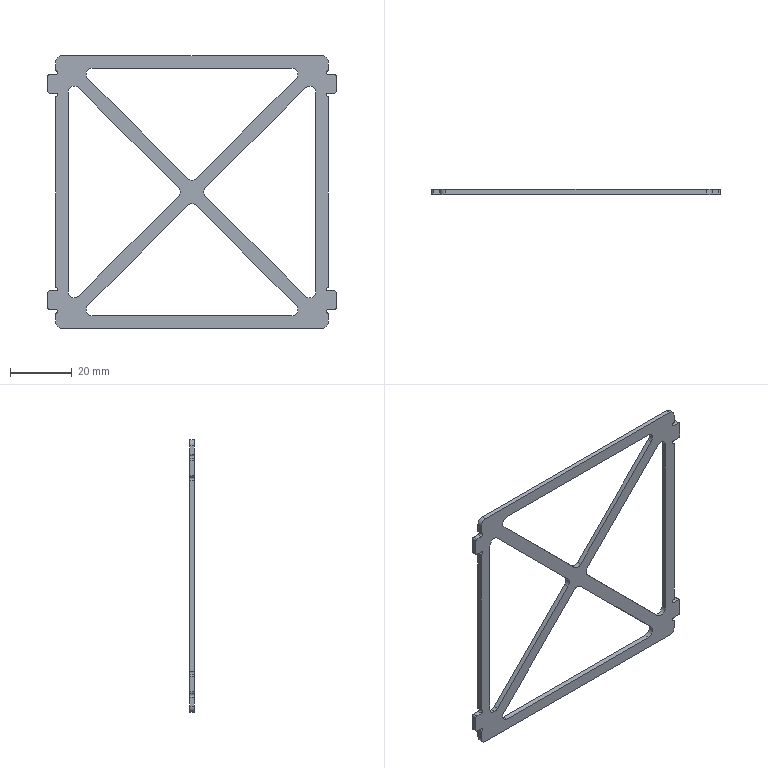Part | SolidWorks | features Fillet 2, Extrusion 1 | 1 solid | 69 faces | box 93.2 x 1.5 x 88.2 mm | volume 3552 mm3 | cylinder 35 | plane 34 | commonest cylinder face diameters 4 x19 1 x8 1.2 x8